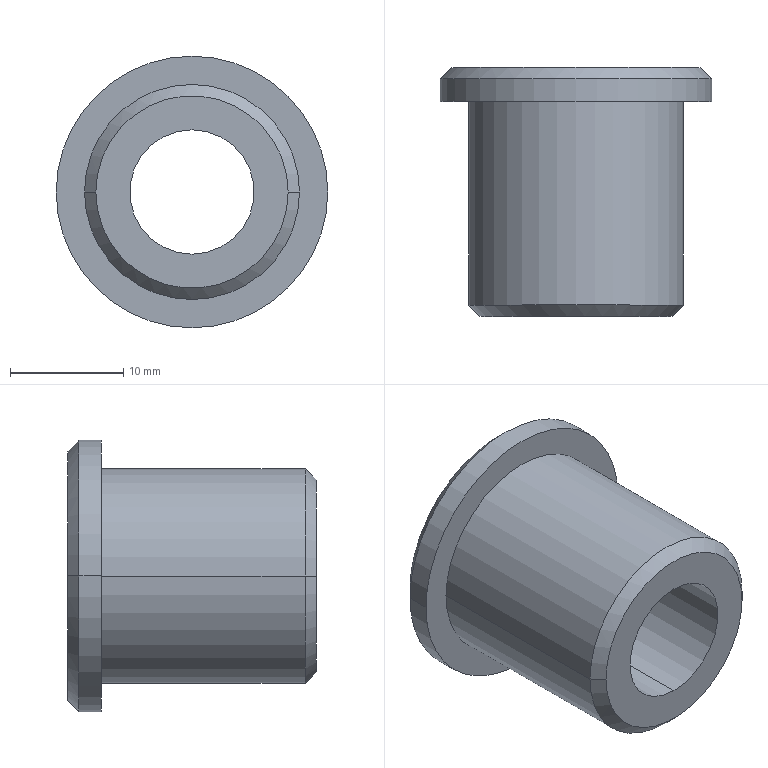Part | SolidWorks | features Chamfer 2, ICE 1, Revolution 1 | 1 solid | 13 faces | box 24 x 22 x 24 mm | volume 4588 mm3 | cylinder 6 | cone 4 | plane 3 | commonest cylinder face diameters 11 x2 19 x2 24 x2
STEP:
#1=CARTESIAN_POINT('',(8.5,0.,0.));
#2=VERTEX_POINT('',#1);
#3=CARTESIAN_POINT('',(-8.5,0.,0.));
#4=VERTEX_POINT('',#3);
#5=CARTESIAN_POINT('',(0.,0.,0.));
#6=DIRECTION('',(0.,-1.,0.));
#7=DIRECTION('',(1.,0.,0.));
#8=AXIS2_PLACEMENT_3D('',#5,#6,#7);
#9=CIRCLE('',#8,8.5);
#10=EDGE_CURVE('',#2,#4,#9,.T.);
#11=ORIENTED_EDGE('',*,*,#10,.F.);
#12=CARTESIAN_POINT('',(9.5,1.,0.));
#13=VERTEX_POINT('',#12);
#14=CARTESIAN_POINT('',(8.5,0.,0.));
#15=DIRECTION('',(0.7071,0.7071,0.));
#16=VECTOR('',#15,1000.);
#17=LINE('',#14,#16);
#18=EDGE_CURVE('',#2,#13,#17,.T.);
#19=ORIENTED_EDGE('',*,*,#18,.T.);
#20=CARTESIAN_POINT('',(-9.5,1.,0.));
#21=VERTEX_POINT('',#20);
#22=CARTESIAN_POINT('',(0.,1.,0.));
#23=DIRECTION('',(0.,1.,0.));
#24=DIRECTION('',(1.,0.,0.));
#25=AXIS2_PLACEMENT_3D('',#22,#23,#24);
#26=CIRCLE('',#25,9.5);
#27=EDGE_CURVE('',#21,#13,#26,.T.);
#28=ORIENTED_EDGE('',*,*,#27,.F.);
#29=CARTESIAN_POINT('',(-8.5,0.,0.));
#30=DIRECTION('',(-0.7071,0.7071,0.));
#31=VECTOR('',#30,1000.);
#32=LINE('',#29,#31);
#33=EDGE_CURVE('',#4,#21,#32,.T.);
#34=ORIENTED_EDGE('',*,*,#33,.F.);
#35=EDGE_LOOP('',(#11,#19,#28,#34));
#36=FACE_OUTER_BOUND('',#35,.T.);
#37=CARTESIAN_POINT('',(0.,0.,0.));
#38=DIRECTION('',(0.,1.,0.));
#39=DIRECTION('',(-1.,0.,0.));
#40=AXIS2_PLACEMENT_3D('',#37,#38,#39);
#41=CONICAL_SURFACE('',#40,8.5,0.7854);
#42=ADVANCED_FACE('',(#36),#41,.T.);
#43=CARTESIAN_POINT('',(-11.,22.,0.));
#44=VERTEX_POINT('',#43);
#45=CARTESIAN_POINT('',(11.,22.,0.));
#46=VERTEX_POINT('',#45);
#47=CARTESIAN_POINT('',(0.,22.,0.));
#48=DIRECTION('',(0.,1.,0.));
#49=DIRECTION('',(-1.,0.,0.));
#50=AXIS2_PLACEMENT_3D('',#47,#48,#49);
#51=CIRCLE('',#50,11.);
#52=EDGE_CURVE('',#44,#46,#51,.T.);
#53=ORIENTED_EDGE('',*,*,#52,.F.);
#54=CARTESIAN_POINT('',(-12.,21.,0.));
#55=VERTEX_POINT('',#54);
#56=CARTESIAN_POINT('',(-12.,21.,0.));
#57=DIRECTION('',(-0.7071,-0.7071,0.));
#58=VECTOR('',#57,1000.);
#59=LINE('',#56,#58);
#60=EDGE_CURVE('',#44,#55,#59,.T.);
#61=ORIENTED_EDGE('',*,*,#60,.T.);
#62=CARTESIAN_POINT('',(12.,21.,0.));
#63=VERTEX_POINT('',#62);
#64=CARTESIAN_POINT('',(0.,21.,0.));
#65=DIRECTION('',(0.,-1.,0.));
#66=DIRECTION('',(-1.,0.,0.));
#67=AXIS2_PLACEMENT_3D('',#64,#65,#66);
#68=CIRCLE('',#67,12.);
#69=EDGE_CURVE('',#63,#55,#68,.T.);
#70=ORIENTED_EDGE('',*,*,#69,.F.);
#71=CARTESIAN_POINT('',(12.,21.,0.));
#72=DIRECTION('',(0.7071,-0.7071,0.));
#73=VECTOR('',#72,1000.);
#74=LINE('',#71,#73);
#75=EDGE_CURVE('',#46,#63,#74,.T.);
#76=ORIENTED_EDGE('',*,*,#75,.F.);
#77=EDGE_LOOP('',(#53,#61,#70,#76));
#78=FACE_OUTER_BOUND('',#77,.T.);
#79=CARTESIAN_POINT('',(0.,21.,0.));
#80=DIRECTION('',(0.,-1.,0.));
#81=DIRECTION('',(1.,0.,0.));
#82=AXIS2_PLACEMENT_3D('',#79,#80,#81);
#83=CONICAL_SURFACE('',#82,12.,0.7854);
#84=ADVANCED_FACE('',(#78),#83,.T.);
#85=CARTESIAN_POINT('',(0.,22.,5.5));
#86=VERTEX_POINT('',#85);
#87=CARTESIAN_POINT('',(0.,22.,-5.5));
#88=VERTEX_POINT('',#87);
#89=CARTESIAN_POINT('',(0.,22.,0.));
#90=DIRECTION('',(0.,-1.,0.));
#91=DIRECTION('',(0.,0.,-1.));
#92=AXIS2_PLACEMENT_3D('',#89,#90,#91);
#93=CIRCLE('',#92,5.5);
#94=EDGE_CURVE('',#86,#88,#93,.T.);
#95=ORIENTED_EDGE('',*,*,#94,.F.);
#96=CARTESIAN_POINT('',(0.,0.,5.5));
#97=VERTEX_POINT('',#96);
#98=CARTESIAN_POINT('',(0.,22.,5.5));
#99=DIRECTION('',(0.,-1.,0.));
#100=VECTOR('',#99,1000.);
#101=LINE('',#98,#100);
#102=EDGE_CURVE('',#86,#97,#101,.T.);
#103=ORIENTED_EDGE('',*,*,#102,.T.);
#104=CARTESIAN_POINT('',(0.,0.,-5.5));
#105=VERTEX_POINT('',#104);
#106=CARTESIAN_POINT('',(0.,0.,0.));
#107=DIRECTION('',(0.,-1.,0.));
#108=DIRECTION('',(0.,0.,-1.));
#109=AXIS2_PLACEMENT_3D('',#106,#107,#108);
#110=CIRCLE('',#109,5.5);
#111=EDGE_CURVE('',#97,#105,#110,.T.);
#112=ORIENTED_EDGE('',*,*,#111,.T.);
#113=CARTESIAN_POINT('',(0.,22.,-5.5));
#114=DIRECTION('',(0.,-1.,0.));
#115=VECTOR('',#114,1000.);
#116=LINE('',#113,#115);
#117=EDGE_CURVE('',#88,#105,#116,.T.);
#118=ORIENTED_EDGE('',*,*,#117,.F.);
#119=EDGE_LOOP('',(#95,#103,#112,#118));
#120=FACE_OUTER_BOUND('',#119,.T.);
#121=CARTESIAN_POINT('',(0.,22.,0.));
#122=DIRECTION('',(0.,-1.,0.));
#123=DIRECTION('',(0.,0.,-1.));
#124=AXIS2_PLACEMENT_3D('',#121,#122,#123);
#125=CYLINDRICAL_SURFACE('',#124,5.5);
#126=ADVANCED_FACE('',(#120),#125,.F.);
#127=CARTESIAN_POINT('',(9.5,19.,0.));
#128=VERTEX_POINT('',#127);
#129=CARTESIAN_POINT('',(-9.5,19.,0.));
#130=VERTEX_POINT('',#129);
#131=CARTESIAN_POINT('',(0.,19.,0.));
#132=DIRECTION('',(0.,-1.,0.));
#133=DIRECTION('',(1.,0.,0.));
#134=AXIS2_PLACEMENT_3D('',#131,#132,#133);
#135=CIRCLE('',#134,9.5);
#136=EDGE_CURVE('',#128,#130,#135,.T.);
#137=ORIENTED_EDGE('',*,*,#136,.T.);
#138=CARTESIAN_POINT('',(-9.5,0.,0.));
#139=DIRECTION('',(0.,-1.,0.));
#140=VECTOR('',#139,1000.);
#141=LINE('',#138,#140);
#142=EDGE_CURVE('',#130,#21,#141,.T.);
#143=ORIENTED_EDGE('',*,*,#142,.T.);
#144=ORIENTED_EDGE('',*,*,#27,.T.);
#145=CARTESIAN_POINT('',(9.5,0.,0.));
#146=DIRECTION('',(0.,-1.,0.));
#147=VECTOR('',#146,1000.);
#148=LINE('',#145,#147);
#149=EDGE_CURVE('',#128,#13,#148,.T.);
#150=ORIENTED_EDGE('',*,*,#149,.F.);
#151=EDGE_LOOP('',(#137,#143,#144,#150));
#152=FACE_OUTER_BOUND('',#151,.T.);
#153=CARTESIAN_POINT('',(0.,0.,0.));
#154=DIRECTION('',(0.,-1.,0.));
#155=DIRECTION('',(1.,0.,0.));
#156=AXIS2_PLACEMENT_3D('',#153,#154,#155);
#157=CYLINDRICAL_SURFACE('',#156,9.5);
#158=ADVANCED_FACE('',(#152),#157,.T.);
#159=ORIENTED_EDGE('',*,*,#69,.T.);
#160=CARTESIAN_POINT('',(-12.,19.,0.));
#161=VERTEX_POINT('',#160);
#162=CARTESIAN_POINT('',(-12.,0.,0.));
#163=DIRECTION('',(0.,-1.,0.));
#164=VECTOR('',#163,1000.);
#165=LINE('',#162,#164);
#166=EDGE_CURVE('',#55,#161,#165,.T.);
#167=ORIENTED_EDGE('',*,*,#166,.T.);
#168=CARTESIAN_POINT('',(12.,19.,0.));
#169=VERTEX_POINT('',#168);
#170=CARTESIAN_POINT('',(0.,19.,0.));
#171=DIRECTION('',(0.,-1.,0.));
#172=DIRECTION('',(1.,0.,0.));
#173=AXIS2_PLACEMENT_3D('',#170,#171,#172);
#174=CIRCLE('',#173,12.);
#175=EDGE_CURVE('',#169,#161,#174,.T.);
#176=ORIENTED_EDGE('',*,*,#175,.F.);
#177=CARTESIAN_POINT('',(12.,0.,0.));
#178=DIRECTION('',(0.,-1.,0.));
#179=VECTOR('',#178,1000.);
#180=LINE('',#177,#179);
#181=EDGE_CURVE('',#63,#169,#180,.T.);
#182=ORIENTED_EDGE('',*,*,#181,.F.);
#183=EDGE_LOOP('',(#159,#167,#176,#182));
#184=FACE_OUTER_BOUND('',#183,.T.);
#185=CARTESIAN_POINT('',(0.,0.,0.));
#186=DIRECTION('',(0.,-1.,0.));
#187=DIRECTION('',(1.,0.,0.));
#188=AXIS2_PLACEMENT_3D('',#185,#186,#187);
#189=CYLINDRICAL_SURFACE('',#188,12.);
#190=ADVANCED_FACE('',(#184),#189,.T.);
#191=CARTESIAN_POINT('',(0.,0.,0.));
#192=DIRECTION('',(0.,-1.,0.));
#193=DIRECTION('',(1.,0.,0.));
#194=AXIS2_PLACEMENT_3D('',#191,#192,#193);
#195=CIRCLE('',#194,8.5);
#196=EDGE_CURVE('',#4,#2,#195,.T.);
#197=ORIENTED_EDGE('',*,*,#196,.T.);
#198=ORIENTED_EDGE('',*,*,#10,.T.);
#199=EDGE_LOOP('',(#197,#198));
#200=FACE_OUTER_BOUND('',#199,.T.);
#201=CARTESIAN_POINT('',(0.,0.,0.));
#202=DIRECTION('',(0.,-1.,0.));
#203=DIRECTION('',(0.,0.,-1.));
#204=AXIS2_PLACEMENT_3D('',#201,#202,#203);
#205=CIRCLE('',#204,5.5);
#206=EDGE_CURVE('',#105,#97,#205,.T.);
#207=ORIENTED_EDGE('',*,*,#206,.F.);
#208=ORIENTED_EDGE('',*,*,#111,.F.);
#209=EDGE_LOOP('',(#207,#208));
#210=FACE_BOUND('',#209,.T.);
#211=CARTESIAN_POINT('',(9.5,0.,0.));
#212=DIRECTION('',(0.,-1.,0.));
#213=DIRECTION('',(1.,0.,0.));
#214=AXIS2_PLACEMENT_3D('',#211,#212,#213);
#215=PLANE('',#214);
#216=ADVANCED_FACE('',(#200,#210),#215,.T.);
#217=CARTESIAN_POINT('',(0.,22.,0.));
#218=DIRECTION('',(0.,1.,0.));
#219=DIRECTION('',(-1.,0.,0.));
#220=AXIS2_PLACEMENT_3D('',#217,#218,#219);
#221=CIRCLE('',#220,11.);
#222=EDGE_CURVE('',#46,#44,#221,.T.);
#223=ORIENTED_EDGE('',*,*,#222,.T.);
#224=ORIENTED_EDGE('',*,*,#52,.T.);
#225=EDGE_LOOP('',(#223,#224));
#226=FACE_OUTER_BOUND('',#225,.T.);
#227=CARTESIAN_POINT('',(0.,22.,0.));
#228=DIRECTION('',(0.,-1.,0.));
#229=DIRECTION('',(0.,0.,-1.));
#230=AXIS2_PLACEMENT_3D('',#227,#228,#229);
#231=CIRCLE('',#230,5.5);
#232=EDGE_CURVE('',#88,#86,#231,.T.);
#233=ORIENTED_EDGE('',*,*,#232,.T.);
#234=ORIENTED_EDGE('',*,*,#94,.T.);
#235=EDGE_LOOP('',(#233,#234));
#236=FACE_BOUND('',#235,.T.);
#237=CARTESIAN_POINT('',(0.,22.,0.));
#238=DIRECTION('',(0.,1.,0.));
#239=DIRECTION('',(-1.,0.,0.));
#240=AXIS2_PLACEMENT_3D('',#237,#238,#239);
#241=PLANE('',#240);
#242=ADVANCED_FACE('',(#226,#236),#241,.T.);
#243=ORIENTED_EDGE('',*,*,#166,.F.);
#244=CARTESIAN_POINT('',(0.,21.,0.));
#245=DIRECTION('',(0.,-1.,0.));
#246=DIRECTION('',(-1.,0.,0.));
#247=AXIS2_PLACEMENT_3D('',#244,#245,#246);
#248=CIRCLE('',#247,12.);
#249=EDGE_CURVE('',#55,#63,#248,.T.);
#250=ORIENTED_EDGE('',*,*,#249,.T.);
#251=ORIENTED_EDGE('',*,*,#181,.T.);
#252=CARTESIAN_POINT('',(0.,19.,0.));
#253=DIRECTION('',(0.,-1.,0.));
#254=DIRECTION('',(1.,0.,0.));
#255=AXIS2_PLACEMENT_3D('',#252,#253,#254);
#256=CIRCLE('',#255,12.);
#257=EDGE_CURVE('',#161,#169,#256,.T.);
#258=ORIENTED_EDGE('',*,*,#257,.F.);
#259=EDGE_LOOP('',(#243,#250,#251,#258));
#260=FACE_OUTER_BOUND('',#259,.T.);
#261=CARTESIAN_POINT('',(0.,0.,0.));
#262=DIRECTION('',(0.,-1.,0.));
#263=DIRECTION('',(1.,0.,0.));
#264=AXIS2_PLACEMENT_3D('',#261,#262,#263);
#265=CYLINDRICAL_SURFACE('',#264,12.);
#266=ADVANCED_FACE('',(#260),#265,.T.);
#267=ORIENTED_EDGE('',*,*,#175,.T.);
#268=ORIENTED_EDGE('',*,*,#257,.T.);
#269=EDGE_LOOP('',(#267,#268));
#270=FACE_OUTER_BOUND('',#269,.T.);
#271=ORIENTED_EDGE('',*,*,#136,.F.);
#272=CARTESIAN_POINT('',(0.,19.,0.));
#273=DIRECTION('',(0.,-1.,0.));
#274=DIRECTION('',(1.,0.,0.));
#275=AXIS2_PLACEMENT_3D('',#272,#273,#274);
#276=CIRCLE('',#275,9.5);
#277=EDGE_CURVE('',#130,#128,#276,.T.);
#278=ORIENTED_EDGE('',*,*,#277,.F.);
#279=EDGE_LOOP('',(#271,#278));
#280=FACE_BOUND('',#279,.T.);
#281=CARTESIAN_POINT('',(12.,19.,0.));
#282=DIRECTION('',(0.,-1.,0.));
#283=DIRECTION('',(1.,0.,0.));
#284=AXIS2_PLACEMENT_3D('',#281,#282,#283);
#285=PLANE('',#284);
#286=ADVANCED_FACE('',(#270,#280),#285,.T.);
#287=ORIENTED_EDGE('',*,*,#142,.F.);
#288=ORIENTED_EDGE('',*,*,#277,.T.);
#289=ORIENTED_EDGE('',*,*,#149,.T.);
#290=CARTESIAN_POINT('',(0.,1.,0.));
#291=DIRECTION('',(0.,1.,0.));
#292=DIRECTION('',(1.,0.,0.));
#293=AXIS2_PLACEMENT_3D('',#290,#291,#292);
#294=CIRCLE('',#293,9.5);
#295=EDGE_CURVE('',#13,#21,#294,.T.);
#296=ORIENTED_EDGE('',*,*,#295,.T.);
#297=EDGE_LOOP('',(#287,#288,#289,#296));
#298=FACE_OUTER_BOUND('',#297,.T.);
#299=CARTESIAN_POINT('',(0.,0.,0.));
#300=DIRECTION('',(0.,-1.,0.));
#301=DIRECTION('',(1.,0.,0.));
#302=AXIS2_PLACEMENT_3D('',#299,#300,#301);
#303=CYLINDRICAL_SURFACE('',#302,9.5);
#304=ADVANCED_FACE('',(#298),#303,.T.);
#305=ORIENTED_EDGE('',*,*,#102,.F.);
#306=ORIENTED_EDGE('',*,*,#232,.F.);
#307=ORIENTED_EDGE('',*,*,#117,.T.);
#308=ORIENTED_EDGE('',*,*,#206,.T.);
#309=EDGE_LOOP('',(#305,#306,#307,#308));
#310=FACE_OUTER_BOUND('',#309,.T.);
#311=CARTESIAN_POINT('',(0.,22.,0.));
#312=DIRECTION('',(0.,-1.,0.));
#313=DIRECTION('',(0.,0.,-1.));
#314=AXIS2_PLACEMENT_3D('',#311,#312,#313);
#315=CYLINDRICAL_SURFACE('',#314,5.5);
#316=ADVANCED_FACE('',(#310),#315,.F.);
#317=ORIENTED_EDGE('',*,*,#60,.F.);
#318=ORIENTED_EDGE('',*,*,#222,.F.);
#319=ORIENTED_EDGE('',*,*,#75,.T.);
#320=ORIENTED_EDGE('',*,*,#249,.F.);
#321=EDGE_LOOP('',(#317,#318,#319,#320));
#322=FACE_OUTER_BOUND('',#321,.T.);
#323=CARTESIAN_POINT('',(0.,21.,0.));
#324=DIRECTION('',(0.,-1.,0.));
#325=DIRECTION('',(1.,0.,0.));
#326=AXIS2_PLACEMENT_3D('',#323,#324,#325);
#327=CONICAL_SURFACE('',#326,12.,0.7854);
#328=ADVANCED_FACE('',(#322),#327,.T.);
#329=ORIENTED_EDGE('',*,*,#18,.F.);
#330=ORIENTED_EDGE('',*,*,#196,.F.);
#331=ORIENTED_EDGE('',*,*,#33,.T.);
#332=ORIENTED_EDGE('',*,*,#295,.F.);
#333=EDGE_LOOP('',(#329,#330,#331,#332));
#334=FACE_OUTER_BOUND('',#333,.T.);
#335=CARTESIAN_POINT('',(0.,0.,0.));
#336=DIRECTION('',(0.,1.,0.));
#337=DIRECTION('',(-1.,0.,0.));
#338=AXIS2_PLACEMENT_3D('',#335,#336,#337);
#339=CONICAL_SURFACE('',#338,8.5,0.7854);
#340=ADVANCED_FACE('',(#334),#339,.T.);
#341=CLOSED_SHELL('',(#42,#84,#126,#158,#190,#216,#242,#266,#286,#304,#316,#328,#340));
#342=MANIFOLD_SOLID_BREP('',#341);
#343=CARTESIAN_POINT('',(0.,0.,0.));
#344=DIRECTION('',(0.,0.,1.));
#345=DIRECTION('',(1.,0.,0.));
#346=AXIS2_PLACEMENT_3D('',#343,#344,#345);
#347=(LENGTH_UNIT()NAMED_UNIT(*)SI_UNIT(.MILLI.,.METRE.));
#348=UNCERTAINTY_MEASURE_WITH_UNIT(LENGTH_MEASURE(0.00001),#347,'','');
#349=(NAMED_UNIT(*)PLANE_ANGLE_UNIT()SI_UNIT($,.RADIAN.));
#350=(NAMED_UNIT(*)SI_UNIT($,.STERADIAN.)SOLID_ANGLE_UNIT());
#351=(GEOMETRIC_REPRESENTATION_CONTEXT(3)GLOBAL_UNCERTAINTY_ASSIGNED_CONTEXT((#348))GLOBAL_UNIT_ASSIGNED_CONTEXT((#347,#349,#350))REPRESENTATION_CONTEXT('',''));
#352=ADVANCED_BREP_SHAPE_REPRESENTATION('',(#342,#346),#351);